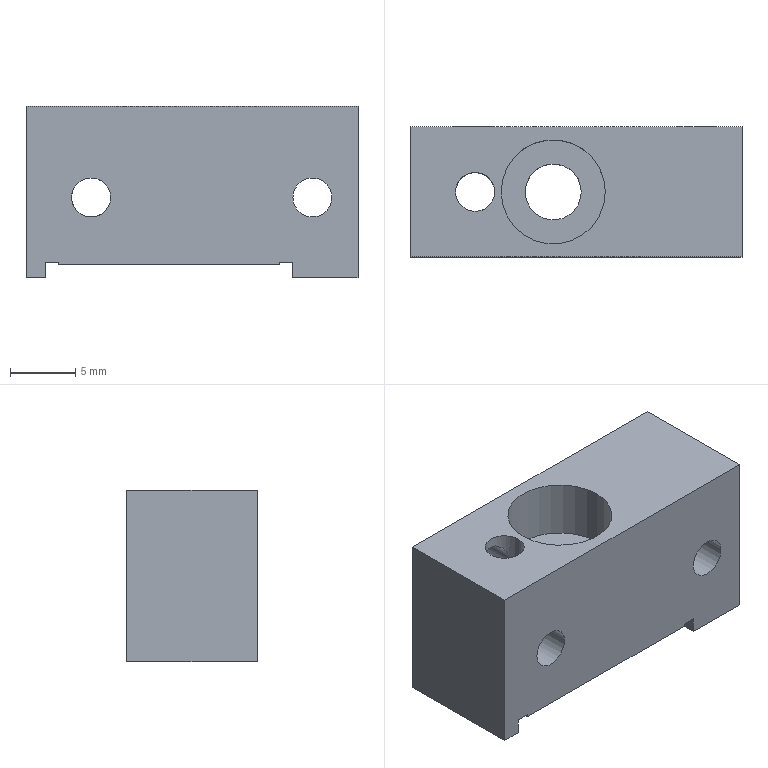Part | NX | 1 solid | 33 faces | box 25.5 x 10 x 13.2 mm | volume 2606 mm3 | cylinder 16 | plane 15 | cone 2 | commonest cylinder face diameters 3 x10 2.5 x2 4.3 x2 8 x2
STEP:
#1=CARTESIAN_POINT('',(9.5,5.,-6.6));
#2=VERTEX_POINT('',#1);
#3=CARTESIAN_POINT('',(9.5,-5.,-6.6));
#4=VERTEX_POINT('',#3);
#5=CARTESIAN_POINT('',(9.5,0.,-6.6));
#6=DIRECTION('',(0.,-1.,0.));
#7=VECTOR('',#6,1000.);
#8=LINE('',#5,#7);
#9=EDGE_CURVE('',#2,#4,#8,.T.);
#10=ORIENTED_EDGE('',*,*,#9,.F.);
#11=CARTESIAN_POINT('',(14.5,5.,-6.6));
#12=VERTEX_POINT('',#11);
#13=CARTESIAN_POINT('',(0.,5.,-6.6));
#14=DIRECTION('',(-1.,0.,0.));
#15=VECTOR('',#14,1000.);
#16=LINE('',#13,#15);
#17=EDGE_CURVE('',#12,#2,#16,.T.);
#18=ORIENTED_EDGE('',*,*,#17,.F.);
#19=CARTESIAN_POINT('',(14.5,-5.,-6.6));
#20=VERTEX_POINT('',#19);
#21=CARTESIAN_POINT('',(14.5,0.,-6.6));
#22=DIRECTION('',(0.,1.,0.));
#23=VECTOR('',#22,1000.);
#24=LINE('',#21,#23);
#25=EDGE_CURVE('',#20,#12,#24,.T.);
#26=ORIENTED_EDGE('',*,*,#25,.F.);
#27=CARTESIAN_POINT('',(0.,-5.,-6.6));
#28=DIRECTION('',(1.,0.,0.));
#29=VECTOR('',#28,1000.);
#30=LINE('',#27,#29);
#31=EDGE_CURVE('',#4,#20,#30,.T.);
#32=ORIENTED_EDGE('',*,*,#31,.F.);
#33=EDGE_LOOP('',(#10,#18,#26,#32));
#34=FACE_BOUND('',#33,.T.);
#35=CARTESIAN_POINT('',(0.,0.,-6.6));
#36=DIRECTION('',(0.,0.,1.));
#37=DIRECTION('',(1.,0.,0.));
#38=AXIS2_PLACEMENT_3D('',#35,#36,#37);
#39=PLANE('',#38);
#40=ADVANCED_FACE('',(#34),#39,.F.);
#41=CARTESIAN_POINT('',(9.5,5.,-5.4));
#42=VERTEX_POINT('',#41);
#43=CARTESIAN_POINT('',(9.5,5.,0.));
#44=DIRECTION('',(0.,0.,1.));
#45=VECTOR('',#44,1000.);
#46=LINE('',#43,#45);
#47=EDGE_CURVE('',#2,#42,#46,.T.);
#48=ORIENTED_EDGE('',*,*,#47,.F.);
#49=ORIENTED_EDGE('',*,*,#9,.T.);
#50=CARTESIAN_POINT('',(9.5,-5.,-5.4));
#51=VERTEX_POINT('',#50);
#52=CARTESIAN_POINT('',(9.5,-5.,0.));
#53=DIRECTION('',(0.,0.,-1.));
#54=VECTOR('',#53,1000.);
#55=LINE('',#52,#54);
#56=EDGE_CURVE('',#51,#4,#55,.T.);
#57=ORIENTED_EDGE('',*,*,#56,.F.);
#58=CARTESIAN_POINT('',(9.5,5.,-5.4));
#59=DIRECTION('',(0.,-1.,0.));
#60=VECTOR('',#59,1000.);
#61=LINE('',#58,#60);
#62=EDGE_CURVE('',#42,#51,#61,.T.);
#63=ORIENTED_EDGE('',*,*,#62,.F.);
#64=EDGE_LOOP('',(#48,#49,#57,#63));
#65=FACE_BOUND('',#64,.T.);
#66=CARTESIAN_POINT('',(9.5,-5.,-6.6));
#67=DIRECTION('',(1.,0.,0.));
#68=DIRECTION('',(0.,1.,0.));
#69=AXIS2_PLACEMENT_3D('',#66,#67,#68);
#70=PLANE('',#69);
#71=ADVANCED_FACE('',(#65),#70,.F.);
#72=CARTESIAN_POINT('',(-11.,-5.,6.6));
#73=VERTEX_POINT('',#72);
#74=CARTESIAN_POINT('',(-11.,5.,6.6));
#75=VERTEX_POINT('',#74);
#76=CARTESIAN_POINT('',(-11.,0.,6.6));
#77=DIRECTION('',(0.,1.,0.));
#78=VECTOR('',#77,1000.);
#79=LINE('',#76,#78);
#80=EDGE_CURVE('',#73,#75,#79,.T.);
#81=ORIENTED_EDGE('',*,*,#80,.F.);
#82=CARTESIAN_POINT('',(14.5,-5.,6.6));
#83=VERTEX_POINT('',#82);
#84=CARTESIAN_POINT('',(0.,-5.,6.6));
#85=DIRECTION('',(-1.,0.,0.));
#86=VECTOR('',#85,1000.);
#87=LINE('',#84,#86);
#88=EDGE_CURVE('',#83,#73,#87,.T.);
#89=ORIENTED_EDGE('',*,*,#88,.F.);
#90=CARTESIAN_POINT('',(14.5,5.,6.6));
#91=VERTEX_POINT('',#90);
#92=CARTESIAN_POINT('',(14.5,0.,6.6));
#93=DIRECTION('',(0.,-1.,0.));
#94=VECTOR('',#93,1000.);
#95=LINE('',#92,#94);
#96=EDGE_CURVE('',#91,#83,#95,.T.);
#97=ORIENTED_EDGE('',*,*,#96,.F.);
#98=CARTESIAN_POINT('',(0.,5.,6.6));
#99=DIRECTION('',(-1.,0.,0.));
#100=VECTOR('',#99,1000.);
#101=LINE('',#98,#100);
#102=EDGE_CURVE('',#91,#75,#101,.T.);
#103=ORIENTED_EDGE('',*,*,#102,.T.);
#104=EDGE_LOOP('',(#81,#89,#97,#103));
#105=FACE_BOUND('',#104,.T.);
#106=CARTESIAN_POINT('',(4.,0.,6.6));
#107=VERTEX_POINT('',#106);
#108=CARTESIAN_POINT('',(-4.,0.,6.6));
#109=VERTEX_POINT('',#108);
#110=CARTESIAN_POINT('',(0.,0.,6.6));
#111=DIRECTION('',(0.,0.,1.));
#112=DIRECTION('',(-1.,0.,0.));
#113=AXIS2_PLACEMENT_3D('',#110,#111,#112);
#114=CIRCLE('',#113,4.);
#115=EDGE_CURVE('',#107,#109,#114,.T.);
#116=ORIENTED_EDGE('',*,*,#115,.F.);
#117=CARTESIAN_POINT('',(0.,0.,6.6));
#118=DIRECTION('',(0.,0.,1.));
#119=DIRECTION('',(-1.,0.,0.));
#120=AXIS2_PLACEMENT_3D('',#117,#118,#119);
#121=CIRCLE('',#120,4.);
#122=EDGE_CURVE('',#109,#107,#121,.T.);
#123=ORIENTED_EDGE('',*,*,#122,.F.);
#124=EDGE_LOOP('',(#116,#123));
#125=FACE_BOUND('',#124,.T.);
#126=CARTESIAN_POINT('',(-4.5,0.,6.6));
#127=VERTEX_POINT('',#126);
#128=CARTESIAN_POINT('',(-7.5,0.,6.6));
#129=VERTEX_POINT('',#128);
#130=CARTESIAN_POINT('',(-6.,0.,6.6));
#131=DIRECTION('',(0.,0.,-1.));
#132=DIRECTION('',(-1.,0.,0.));
#133=AXIS2_PLACEMENT_3D('',#130,#131,#132);
#134=CIRCLE('',#133,1.5);
#135=EDGE_CURVE('',#127,#129,#134,.T.);
#136=ORIENTED_EDGE('',*,*,#135,.T.);
#137=CARTESIAN_POINT('',(-6.,0.,6.6));
#138=DIRECTION('',(0.,0.,-1.));
#139=DIRECTION('',(-1.,0.,0.));
#140=AXIS2_PLACEMENT_3D('',#137,#138,#139);
#141=CIRCLE('',#140,1.5);
#142=EDGE_CURVE('',#129,#127,#141,.T.);
#143=ORIENTED_EDGE('',*,*,#142,.T.);
#144=EDGE_LOOP('',(#136,#143));
#145=FACE_BOUND('',#144,.T.);
#146=CARTESIAN_POINT('',(0.,0.,6.6));
#147=DIRECTION('',(0.,0.,1.));
#148=DIRECTION('',(1.,0.,0.));
#149=AXIS2_PLACEMENT_3D('',#146,#147,#148);
#150=PLANE('',#149);
#151=ADVANCED_FACE('',(#105,#125,#145),#150,.T.);
#152=CARTESIAN_POINT('',(8.5,-5.,-5.4));
#153=VERTEX_POINT('',#152);
#154=CARTESIAN_POINT('',(0.,-5.,-5.4));
#155=DIRECTION('',(1.,0.,0.));
#156=VECTOR('',#155,1000.);
#157=LINE('',#154,#156);
#158=EDGE_CURVE('',#153,#51,#157,.T.);
#159=ORIENTED_EDGE('',*,*,#158,.F.);
#160=CARTESIAN_POINT('',(8.5,5.,-5.4));
#161=VERTEX_POINT('',#160);
#162=CARTESIAN_POINT('',(8.5,5.,-5.4));
#163=DIRECTION('',(0.,-1.,0.));
#164=VECTOR('',#163,1000.);
#165=LINE('',#162,#164);
#166=EDGE_CURVE('',#161,#153,#165,.T.);
#167=ORIENTED_EDGE('',*,*,#166,.F.);
#168=CARTESIAN_POINT('',(0.,5.,-5.4));
#169=DIRECTION('',(-1.,0.,0.));
#170=VECTOR('',#169,1000.);
#171=LINE('',#168,#170);
#172=EDGE_CURVE('',#42,#161,#171,.T.);
#173=ORIENTED_EDGE('',*,*,#172,.F.);
#174=ORIENTED_EDGE('',*,*,#62,.T.);
#175=EDGE_LOOP('',(#159,#167,#173,#174));
#176=FACE_BOUND('',#175,.T.);
#177=CARTESIAN_POINT('',(9.5,-5.,-5.4));
#178=DIRECTION('',(0.,0.,1.));
#179=DIRECTION('',(1.,0.,0.));
#180=AXIS2_PLACEMENT_3D('',#177,#178,#179);
#181=PLANE('',#180);
#182=ADVANCED_FACE('',(#176),#181,.F.);
#183=CARTESIAN_POINT('',(-7.5,0.,-0.42));
#184=VERTEX_POINT('',#183);
#185=CARTESIAN_POINT('',(-4.5,0.,-0.42));
#186=VERTEX_POINT('',#185);
#187=CARTESIAN_POINT('',(-7.5,0.,-0.42));
#188=CARTESIAN_POINT('',(-7.5,3.,-3.42));
#189=CARTESIAN_POINT('',(-4.5,3.,-3.42));
#190=CARTESIAN_POINT('',(-4.5,0.,-0.42));
#191=(BOUNDED_CURVE()B_SPLINE_CURVE(3,(#187,#188,#189,#190),.UNSPECIFIED.,.F.,.F.)B_SPLINE_CURVE_WITH_KNOTS((4,4),(4.712,7.854),.UNSPECIFIED.)CURVE()GEOMETRIC_REPRESENTATION_ITEM()RATIONAL_B_SPLINE_CURVE((1.,0.3333,0.3333,1.))REPRESENTATION_ITEM(''));
#192=EDGE_CURVE('',#184,#186,#191,.T.);
#193=ORIENTED_EDGE('',*,*,#192,.F.);
#194=CARTESIAN_POINT('',(-7.5,0.,-5.6));
#195=VERTEX_POINT('',#194);
#196=CARTESIAN_POINT('',(-7.5,0.,6.6));
#197=DIRECTION('',(0.,0.,-1.));
#198=VECTOR('',#197,1000.);
#199=LINE('',#196,#198);
#200=EDGE_CURVE('',#195,#184,#199,.F.);
#201=ORIENTED_EDGE('',*,*,#200,.F.);
#202=CARTESIAN_POINT('',(-4.5,0.,-5.6));
#203=VERTEX_POINT('',#202);
#204=CARTESIAN_POINT('',(-6.,0.,-5.6));
#205=DIRECTION('',(0.,0.,-1.));
#206=DIRECTION('',(-1.,0.,0.));
#207=AXIS2_PLACEMENT_3D('',#204,#205,#206);
#208=CIRCLE('',#207,1.5);
#209=EDGE_CURVE('',#195,#203,#208,.T.);
#210=ORIENTED_EDGE('',*,*,#209,.T.);
#211=CARTESIAN_POINT('',(-4.5,0.,6.6));
#212=DIRECTION('',(0.,0.,-1.));
#213=VECTOR('',#212,1000.);
#214=LINE('',#211,#213);
#215=EDGE_CURVE('',#203,#186,#214,.F.);
#216=ORIENTED_EDGE('',*,*,#215,.T.);
#217=EDGE_LOOP('',(#193,#201,#210,#216));
#218=FACE_BOUND('',#217,.T.);
#219=CARTESIAN_POINT('',(-6.,0.,6.6));
#220=DIRECTION('',(0.,0.,-1.));
#221=DIRECTION('',(-1.,0.,0.));
#222=AXIS2_PLACEMENT_3D('',#219,#220,#221);
#223=CYLINDRICAL_SURFACE('',#222,1.5);
#224=ADVANCED_FACE('',(#218),#223,.F.);
#225=CARTESIAN_POINT('',(-4.5,5.,-0.42));
#226=VERTEX_POINT('',#225);
#227=CARTESIAN_POINT('',(-7.5,5.,-0.42));
#228=VERTEX_POINT('',#227);
#229=CARTESIAN_POINT('',(-6.,5.,-0.42));
#230=DIRECTION('',(0.,1.,0.));
#231=DIRECTION('',(-1.,0.,0.));
#232=AXIS2_PLACEMENT_3D('',#229,#230,#231);
#233=CIRCLE('',#232,1.5);
#234=EDGE_CURVE('',#226,#228,#233,.T.);
#235=ORIENTED_EDGE('',*,*,#234,.T.);
#236=CARTESIAN_POINT('',(-7.5,-5.,-0.42));
#237=DIRECTION('',(0.,1.,0.));
#238=VECTOR('',#237,1000.);
#239=LINE('',#236,#238);
#240=EDGE_CURVE('',#228,#184,#239,.F.);
#241=ORIENTED_EDGE('',*,*,#240,.T.);
#242=ORIENTED_EDGE('',*,*,#192,.T.);
#243=CARTESIAN_POINT('',(-4.5,-5.,-0.42));
#244=DIRECTION('',(0.,1.,0.));
#245=VECTOR('',#244,1000.);
#246=LINE('',#243,#245);
#247=EDGE_CURVE('',#226,#186,#246,.F.);
#248=ORIENTED_EDGE('',*,*,#247,.F.);
#249=EDGE_LOOP('',(#235,#241,#242,#248));
#250=FACE_BOUND('',#249,.T.);
#251=CARTESIAN_POINT('',(-6.,-5.,-0.42));
#252=DIRECTION('',(0.,1.,0.));
#253=DIRECTION('',(-1.,0.,0.));
#254=AXIS2_PLACEMENT_3D('',#251,#252,#253);
#255=CYLINDRICAL_SURFACE('',#254,1.5);
#256=ADVANCED_FACE('',(#250),#255,.F.);
#257=CARTESIAN_POINT('',(9.5,-5.,-0.42));
#258=VERTEX_POINT('',#257);
#259=CARTESIAN_POINT('',(12.5,-5.,-0.42));
#260=VERTEX_POINT('',#259);
#261=CARTESIAN_POINT('',(11.,-5.,-0.42));
#262=DIRECTION('',(0.,1.,0.));
#263=DIRECTION('',(-1.,0.,0.));
#264=AXIS2_PLACEMENT_3D('',#261,#262,#263);
#265=CIRCLE('',#264,1.5);
#266=EDGE_CURVE('',#258,#260,#265,.T.);
#267=ORIENTED_EDGE('',*,*,#266,.F.);
#268=CARTESIAN_POINT('',(9.5,5.,-0.42));
#269=VERTEX_POINT('',#268);
#270=CARTESIAN_POINT('',(9.5,-5.,-0.42));
#271=DIRECTION('',(0.,1.,0.));
#272=VECTOR('',#271,1000.);
#273=LINE('',#270,#272);
#274=EDGE_CURVE('',#269,#258,#273,.F.);
#275=ORIENTED_EDGE('',*,*,#274,.F.);
#276=CARTESIAN_POINT('',(12.5,5.,-0.42));
#277=VERTEX_POINT('',#276);
#278=CARTESIAN_POINT('',(11.,5.,-0.42));
#279=DIRECTION('',(0.,1.,0.));
#280=DIRECTION('',(-1.,0.,0.));
#281=AXIS2_PLACEMENT_3D('',#278,#279,#280);
#282=CIRCLE('',#281,1.5);
#283=EDGE_CURVE('',#269,#277,#282,.T.);
#284=ORIENTED_EDGE('',*,*,#283,.T.);
#285=CARTESIAN_POINT('',(12.5,-5.,-0.42));
#286=DIRECTION('',(0.,1.,0.));
#287=VECTOR('',#286,1000.);
#288=LINE('',#285,#287);
#289=EDGE_CURVE('',#277,#260,#288,.F.);
#290=ORIENTED_EDGE('',*,*,#289,.T.);
#291=EDGE_LOOP('',(#267,#275,#284,#290));
#292=FACE_BOUND('',#291,.T.);
#293=CARTESIAN_POINT('',(11.,-5.,-0.42));
#294=DIRECTION('',(0.,1.,0.));
#295=DIRECTION('',(-1.,0.,0.));
#296=AXIS2_PLACEMENT_3D('',#293,#294,#295);
#297=CYLINDRICAL_SURFACE('',#296,1.5);
#298=ADVANCED_FACE('',(#292),#297,.F.);
#299=ORIENTED_EDGE('',*,*,#135,.F.);
#300=CARTESIAN_POINT('',(-4.5,0.,6.6));
#301=DIRECTION('',(0.,0.,-1.));
#302=VECTOR('',#301,1000.);
#303=LINE('',#300,#302);
#304=EDGE_CURVE('',#186,#127,#303,.F.);
#305=ORIENTED_EDGE('',*,*,#304,.F.);
#306=CARTESIAN_POINT('',(-7.5,0.,-0.42));
#307=CARTESIAN_POINT('',(-7.5,-3.,2.58));
#308=CARTESIAN_POINT('',(-4.5,-3.,2.58));
#309=CARTESIAN_POINT('',(-4.5,0.,-0.42));
#310=(BOUNDED_CURVE()B_SPLINE_CURVE(3,(#306,#307,#308,#309),.UNSPECIFIED.,.F.,.F.)B_SPLINE_CURVE_WITH_KNOTS((4,4),(1.571,4.712),.UNSPECIFIED.)CURVE()GEOMETRIC_REPRESENTATION_ITEM()RATIONAL_B_SPLINE_CURVE((1.,0.3333,0.3333,1.))REPRESENTATION_ITEM(''));
#311=EDGE_CURVE('',#184,#186,#310,.T.);
#312=ORIENTED_EDGE('',*,*,#311,.F.);
#313=CARTESIAN_POINT('',(-7.5,0.,6.6));
#314=DIRECTION('',(0.,0.,-1.));
#315=VECTOR('',#314,1000.);
#316=LINE('',#313,#315);
#317=EDGE_CURVE('',#184,#129,#316,.F.);
#318=ORIENTED_EDGE('',*,*,#317,.T.);
#319=EDGE_LOOP('',(#299,#305,#312,#318));
#320=FACE_BOUND('',#319,.T.);
#321=CARTESIAN_POINT('',(-6.,0.,6.6));
#322=DIRECTION('',(0.,0.,-1.));
#323=DIRECTION('',(-1.,0.,0.));
#324=AXIS2_PLACEMENT_3D('',#321,#322,#323);
#325=CYLINDRICAL_SURFACE('',#324,1.5);
#326=ADVANCED_FACE('',(#320),#325,.F.);
#327=CARTESIAN_POINT('',(-8.5,-5.,-5.6));
#328=VERTEX_POINT('',#327);
#329=CARTESIAN_POINT('',(8.5,-5.,-5.6));
#330=VERTEX_POINT('',#329);
#331=CARTESIAN_POINT('',(0.,-5.,-5.6));
#332=DIRECTION('',(1.,0.,0.));
#333=VECTOR('',#332,1000.);
#334=LINE('',#331,#333);
#335=EDGE_CURVE('',#328,#330,#334,.T.);
#336=ORIENTED_EDGE('',*,*,#335,.T.);
#337=CARTESIAN_POINT('',(8.5,-5.,0.));
#338=DIRECTION('',(0.,0.,1.));
#339=VECTOR('',#338,1000.);
#340=LINE('',#337,#339);
#341=EDGE_CURVE('',#330,#153,#340,.T.);
#342=ORIENTED_EDGE('',*,*,#341,.T.);
#343=ORIENTED_EDGE('',*,*,#158,.T.);
#344=ORIENTED_EDGE('',*,*,#56,.T.);
#345=ORIENTED_EDGE('',*,*,#31,.T.);
#346=CARTESIAN_POINT('',(14.5,-5.,0.));
#347=DIRECTION('',(0.,0.,-1.));
#348=VECTOR('',#347,1000.);
#349=LINE('',#346,#348);
#350=EDGE_CURVE('',#83,#20,#349,.T.);
#351=ORIENTED_EDGE('',*,*,#350,.F.);
#352=ORIENTED_EDGE('',*,*,#88,.T.);
#353=CARTESIAN_POINT('',(-11.,-5.,-6.6));
#354=VERTEX_POINT('',#353);
#355=CARTESIAN_POINT('',(-11.,-5.,0.));
#356=DIRECTION('',(0.,0.,1.));
#357=VECTOR('',#356,1000.);
#358=LINE('',#355,#357);
#359=EDGE_CURVE('',#354,#73,#358,.T.);
#360=ORIENTED_EDGE('',*,*,#359,.F.);
#361=CARTESIAN_POINT('',(-9.5,-5.,-6.6));
#362=VERTEX_POINT('',#361);
#363=CARTESIAN_POINT('',(0.,-5.,-6.6));
#364=DIRECTION('',(1.,0.,0.));
#365=VECTOR('',#364,1000.);
#366=LINE('',#363,#365);
#367=EDGE_CURVE('',#354,#362,#366,.T.);
#368=ORIENTED_EDGE('',*,*,#367,.T.);
#369=CARTESIAN_POINT('',(-9.5,-5.,-5.4));
#370=VERTEX_POINT('',#369);
#371=CARTESIAN_POINT('',(-9.5,-5.,0.));
#372=DIRECTION('',(0.,0.,1.));
#373=VECTOR('',#372,1000.);
#374=LINE('',#371,#373);
#375=EDGE_CURVE('',#362,#370,#374,.T.);
#376=ORIENTED_EDGE('',*,*,#375,.T.);
#377=CARTESIAN_POINT('',(-8.5,-5.,-5.4));
#378=VERTEX_POINT('',#377);
#379=CARTESIAN_POINT('',(0.,-5.,-5.4));
#380=DIRECTION('',(1.,0.,0.));
#381=VECTOR('',#380,1000.);
#382=LINE('',#379,#381);
#383=EDGE_CURVE('',#370,#378,#382,.T.);
#384=ORIENTED_EDGE('',*,*,#383,.T.);
#385=CARTESIAN_POINT('',(-8.5,-5.,0.));
#386=DIRECTION('',(0.,0.,-1.));
#387=VECTOR('',#386,1000.);
#388=LINE('',#385,#387);
#389=EDGE_CURVE('',#378,#328,#388,.T.);
#390=ORIENTED_EDGE('',*,*,#389,.T.);
#391=EDGE_LOOP('',(#336,#342,#343,#344,#345,#351,#352,#360,#368,#376,#384,#390));
#392=FACE_BOUND('',#391,.T.);
#393=CARTESIAN_POINT('',(-4.5,-5.,-0.42));
#394=VERTEX_POINT('',#393);
#395=CARTESIAN_POINT('',(-7.5,-5.,-0.42));
#396=VERTEX_POINT('',#395);
#397=CARTESIAN_POINT('',(-6.,-5.,-0.42));
#398=DIRECTION('',(0.,1.,0.));
#399=DIRECTION('',(-1.,0.,0.));
#400=AXIS2_PLACEMENT_3D('',#397,#398,#399);
#401=CIRCLE('',#400,1.5);
#402=EDGE_CURVE('',#394,#396,#401,.T.);
#403=ORIENTED_EDGE('',*,*,#402,.T.);
#404=CARTESIAN_POINT('',(-6.,-5.,-0.42));
#405=DIRECTION('',(0.,1.,0.));
#406=DIRECTION('',(-1.,0.,0.));
#407=AXIS2_PLACEMENT_3D('',#404,#405,#406);
#408=CIRCLE('',#407,1.5);
#409=EDGE_CURVE('',#396,#394,#408,.T.);
#410=ORIENTED_EDGE('',*,*,#409,.T.);
#411=EDGE_LOOP('',(#403,#410));
#412=FACE_BOUND('',#411,.T.);
#413=ORIENTED_EDGE('',*,*,#266,.T.);
#414=CARTESIAN_POINT('',(11.,-5.,-0.42));
#415=DIRECTION('',(0.,1.,0.));
#416=DIRECTION('',(-1.,0.,0.));
#417=AXIS2_PLACEMENT_3D('',#414,#415,#416);
#418=CIRCLE('',#417,1.5);
#419=EDGE_CURVE('',#260,#258,#418,.T.);
#420=ORIENTED_EDGE('',*,*,#419,.T.);
#421=EDGE_LOOP('',(#413,#420));
#422=FACE_BOUND('',#421,.T.);
#423=CARTESIAN_POINT('',(-11.,-5.,-6.6));
#424=DIRECTION('',(0.,-1.,0.));
#425=DIRECTION('',(0.,0.,-1.));
#426=AXIS2_PLACEMENT_3D('',#423,#424,#425);
#427=PLANE('',#426);
#428=ADVANCED_FACE('',(#392,#412,#422),#427,.T.);
#429=CARTESIAN_POINT('',(-11.,5.,-6.6));
#430=VERTEX_POINT('',#429);
#431=CARTESIAN_POINT('',(-11.,-5.,-6.6));
#432=DIRECTION('',(0.,1.,0.));
#433=VECTOR('',#432,1000.);
#434=LINE('',#431,#433);
#435=EDGE_CURVE('',#354,#430,#434,.T.);
#436=ORIENTED_EDGE('',*,*,#435,.F.);
#437=ORIENTED_EDGE('',*,*,#359,.T.);
#438=ORIENTED_EDGE('',*,*,#80,.T.);
#439=CARTESIAN_POINT('',(-11.,5.,0.));
#440=DIRECTION('',(0.,0.,-1.));
#441=VECTOR('',#440,1000.);
#442=LINE('',#439,#441);
#443=EDGE_CURVE('',#75,#430,#442,.T.);
#444=ORIENTED_EDGE('',*,*,#443,.T.);
#445=EDGE_LOOP('',(#436,#437,#438,#444));
#446=FACE_BOUND('',#445,.T.);
#447=CARTESIAN_POINT('',(-11.,5.,-6.6));
#448=DIRECTION('',(-1.,0.,0.));
#449=DIRECTION('',(0.,0.,1.));
#450=AXIS2_PLACEMENT_3D('',#447,#448,#449);
#451=PLANE('',#450);
#452=ADVANCED_FACE('',(#446),#451,.T.);
#453=CARTESIAN_POINT('',(-9.5,5.,-6.6));
#454=VERTEX_POINT('',#453);
#455=CARTESIAN_POINT('',(-9.5,0.,-6.6));
#456=DIRECTION('',(0.,-1.,0.));
#457=VECTOR('',#456,1000.);
#458=LINE('',#455,#457);
#459=EDGE_CURVE('',#454,#362,#458,.T.);
#460=ORIENTED_EDGE('',*,*,#459,.T.);
#461=ORIENTED_EDGE('',*,*,#367,.F.);
#462=ORIENTED_EDGE('',*,*,#435,.T.);
#463=CARTESIAN_POINT('',(0.,5.,-6.6));
#464=DIRECTION('',(-1.,0.,0.));
#465=VECTOR('',#464,1000.);
#466=LINE('',#463,#465);
#467=EDGE_CURVE('',#454,#430,#466,.T.);
#468=ORIENTED_EDGE('',*,*,#467,.F.);
#469=EDGE_LOOP('',(#460,#461,#462,#468));
#470=FACE_BOUND('',#469,.T.);
#471=CARTESIAN_POINT('',(0.,0.,-6.6));
#472=DIRECTION('',(0.,0.,1.));
#473=DIRECTION('',(1.,0.,0.));
#474=AXIS2_PLACEMENT_3D('',#471,#472,#473);
#475=PLANE('',#474);
#476=ADVANCED_FACE('',(#470),#475,.F.);
#477=ORIENTED_EDGE('',*,*,#375,.F.);
#478=ORIENTED_EDGE('',*,*,#459,.F.);
#479=CARTESIAN_POINT('',(-9.5,5.,-5.4));
#480=VERTEX_POINT('',#479);
#481=CARTESIAN_POINT('',(-9.5,5.,0.));
#482=DIRECTION('',(0.,0.,-1.));
#483=VECTOR('',#482,1000.);
#484=LINE('',#481,#483);
#485=EDGE_CURVE('',#480,#454,#484,.T.);
#486=ORIENTED_EDGE('',*,*,#485,.F.);
#487=CARTESIAN_POINT('',(-9.5,6.,-5.4));
#488=DIRECTION('',(0.,-1.,0.));
#489=VECTOR('',#488,1000.);
#490=LINE('',#487,#489);
#491=EDGE_CURVE('',#480,#370,#490,.T.);
#492=ORIENTED_EDGE('',*,*,#491,.T.);
#493=EDGE_LOOP('',(#477,#478,#486,#492));
#494=FACE_BOUND('',#493,.T.);
#495=CARTESIAN_POINT('',(-9.5,-5.,-5.6));
#496=DIRECTION('',(-1.,0.,0.));
#497=DIRECTION('',(0.,0.,1.));
#498=AXIS2_PLACEMENT_3D('',#495,#496,#497);
#499=PLANE('',#498);
#500=ADVANCED_FACE('',(#494),#499,.F.);
#501=CARTESIAN_POINT('',(-8.5,5.,-5.6));
#502=VERTEX_POINT('',#501);
#503=CARTESIAN_POINT('',(-8.5,0.,-5.6));
#504=DIRECTION('',(0.,-1.,0.));
#505=VECTOR('',#504,1000.);
#506=LINE('',#503,#505);
#507=EDGE_CURVE('',#502,#328,#506,.T.);
#508=ORIENTED_EDGE('',*,*,#507,.F.);
#509=CARTESIAN_POINT('',(8.5,5.,-5.6));
#510=VERTEX_POINT('',#509);
#511=CARTESIAN_POINT('',(0.,5.,-5.6));
#512=DIRECTION('',(-1.,0.,0.));
#513=VECTOR('',#512,1000.);
#514=LINE('',#511,#513);
#515=EDGE_CURVE('',#510,#502,#514,.T.);
#516=ORIENTED_EDGE('',*,*,#515,.F.);
#517=CARTESIAN_POINT('',(8.5,0.,-5.6));
#518=DIRECTION('',(0.,1.,0.));
#519=VECTOR('',#518,1000.);
#520=LINE('',#517,#519);
#521=EDGE_CURVE('',#330,#510,#520,.T.);
#522=ORIENTED_EDGE('',*,*,#521,.F.);
#523=ORIENTED_EDGE('',*,*,#335,.F.);
#524=EDGE_LOOP('',(#508,#516,#522,#523));
#525=FACE_BOUND('',#524,.T.);
#526=CARTESIAN_POINT('',(2.15,0.,-5.6));
#527=VERTEX_POINT('',#526);
#528=CARTESIAN_POINT('',(-2.15,0.,-5.6));
#529=VERTEX_POINT('',#528);
#530=CARTESIAN_POINT('',(0.,0.,-5.6));
#531=DIRECTION('',(0.,0.,1.));
#532=DIRECTION('',(-1.,0.,0.));
#533=AXIS2_PLACEMENT_3D('',#530,#531,#532);
#534=CIRCLE('',#533,2.15);
#535=EDGE_CURVE('',#527,#529,#534,.T.);
#536=ORIENTED_EDGE('',*,*,#535,.T.);
#537=CARTESIAN_POINT('',(0.,0.,-5.6));
#538=DIRECTION('',(0.,0.,1.));
#539=DIRECTION('',(-1.,0.,0.));
#540=AXIS2_PLACEMENT_3D('',#537,#538,#539);
#541=CIRCLE('',#540,2.15);
#542=EDGE_CURVE('',#529,#527,#541,.T.);
#543=ORIENTED_EDGE('',*,*,#542,.T.);
#544=EDGE_LOOP('',(#536,#543));
#545=FACE_BOUND('',#544,.T.);
#546=CARTESIAN_POINT('',(-6.,0.,-5.6));
#547=DIRECTION('',(0.,0.,-1.));
#548=DIRECTION('',(-1.,0.,0.));
#549=AXIS2_PLACEMENT_3D('',#546,#547,#548);
#550=CIRCLE('',#549,1.5);
#551=EDGE_CURVE('',#203,#195,#550,.T.);
#552=ORIENTED_EDGE('',*,*,#551,.F.);
#553=ORIENTED_EDGE('',*,*,#209,.F.);
#554=EDGE_LOOP('',(#552,#553));
#555=FACE_BOUND('',#554,.T.);
#556=CARTESIAN_POINT('',(9.5,-5.,-5.6));
#557=DIRECTION('',(0.,0.,1.));
#558=DIRECTION('',(1.,0.,0.));
#559=AXIS2_PLACEMENT_3D('',#556,#557,#558);
#560=PLANE('',#559);
#561=ADVANCED_FACE('',(#525,#545,#555),#560,.F.);
#562=CARTESIAN_POINT('',(-4.75,0.8292,4.6));
#563=VERTEX_POINT('',#562);
#564=CARTESIAN_POINT('',(-7.25,0.8292,4.6));
#565=VERTEX_POINT('',#564);
#566=CARTESIAN_POINT('',(-4.75,0.8292,4.6));
#567=CARTESIAN_POINT('',(-4.75,0.8292,4.766));
#568=CARTESIAN_POINT('',(-4.828,0.9361,5.054));
#569=CARTESIAN_POINT('',(-4.907,1.037,5.23));
#570=CARTESIAN_POINT('',(-5.078,1.185,5.448));
#571=CARTESIAN_POINT('',(-5.098,1.2,5.467));
#572=CARTESIAN_POINT('',(-5.321,1.346,5.664));
#573=CARTESIAN_POINT('',(-5.543,1.438,5.773));
#574=CARTESIAN_POINT('',(-6.,1.542,5.901));
#575=CARTESIAN_POINT('',(-6.457,1.438,5.774));
#576=CARTESIAN_POINT('',(-6.68,1.345,5.663));
#577=CARTESIAN_POINT('',(-6.9,1.202,5.47));
#578=CARTESIAN_POINT('',(-6.925,1.182,5.444));
#579=CARTESIAN_POINT('',(-7.09,1.039,5.233));
#580=CARTESIAN_POINT('',(-7.174,0.9344,5.052));
#581=CARTESIAN_POINT('',(-7.25,0.8292,4.766));
#582=CARTESIAN_POINT('',(-7.25,0.8292,4.6));
#583=B_SPLINE_CURVE_WITH_KNOTS('',3,(#566,#567,#568,#569,#570,#571,#572,#573,#574,#575,#576,#577,#578,#579,#580,#581,#582),.UNSPECIFIED.,.F.,.F.,(4,1,1,1,1,1,1,1,1,1,1,1,1,1,4),(0.,0.125,0.1875,0.2188,0.25,0.3125,0.375,0.5,0.625,0.6875,0.75,0.7812,0.8125,0.875,1.),.UNSPECIFIED.);
#584=EDGE_CURVE('',#563,#565,#583,.T.);
#585=ORIENTED_EDGE('',*,*,#584,.T.);
#586=CARTESIAN_POINT('',(-7.25,4.74,4.6));
#587=VERTEX_POINT('',#586);
#588=CARTESIAN_POINT('',(-7.25,2.915,4.6));
#589=DIRECTION('',(0.,1.,0.));
#590=VECTOR('',#589,1000.);
#591=LINE('',#588,#590);
#592=EDGE_CURVE('',#587,#565,#591,.F.);
#593=ORIENTED_EDGE('',*,*,#592,.F.);
#594=CARTESIAN_POINT('',(-4.75,4.74,4.6));
#595=VERTEX_POINT('',#594);
#596=CARTESIAN_POINT('',(-6.,4.74,4.6));
#597=DIRECTION('',(0.,1.,0.));
#598=DIRECTION('',(1.,0.,0.));
#599=AXIS2_PLACEMENT_3D('',#596,#597,#598);
#600=CIRCLE('',#599,1.25);
#601=EDGE_CURVE('',#587,#595,#600,.T.);
#602=ORIENTED_EDGE('',*,*,#601,.T.);
#603=CARTESIAN_POINT('',(-4.75,2.915,4.6));
#604=DIRECTION('',(0.,1.,0.));
#605=VECTOR('',#604,1000.);
#606=LINE('',#603,#605);
#607=EDGE_CURVE('',#595,#563,#606,.F.);
#608=ORIENTED_EDGE('',*,*,#607,.T.);
#609=EDGE_LOOP('',(#585,#593,#602,#608));
#610=FACE_BOUND('',#609,.T.);
#611=CARTESIAN_POINT('',(-6.,2.915,4.6));
#612=DIRECTION('',(0.,1.,0.));
#613=DIRECTION('',(-1.,0.,0.));
#614=AXIS2_PLACEMENT_3D('',#611,#612,#613);
#615=CYLINDRICAL_SURFACE('',#614,1.25);
#616=ADVANCED_FACE('',(#610),#615,.F.);
#617=ORIENTED_EDGE('',*,*,#115,.T.);
#618=CARTESIAN_POINT('',(-4.,0.,2.1));
#619=VERTEX_POINT('',#618);
#620=CARTESIAN_POINT('',(-4.,0.,-8.646));
#621=DIRECTION('',(0.,0.,1.));
#622=VECTOR('',#621,1000.);
#623=LINE('',#620,#622);
#624=EDGE_CURVE('',#109,#619,#623,.F.);
#625=ORIENTED_EDGE('',*,*,#624,.T.);
#626=CARTESIAN_POINT('',(4.,0.,2.1));
#627=VERTEX_POINT('',#626);
#628=CARTESIAN_POINT('',(0.,0.,2.1));
#629=DIRECTION('',(0.,0.,-1.));
#630=DIRECTION('',(-1.,0.,0.));
#631=AXIS2_PLACEMENT_3D('',#628,#629,#630);
#632=CIRCLE('',#631,4.);
#633=EDGE_CURVE('',#619,#627,#632,.T.);
#634=ORIENTED_EDGE('',*,*,#633,.T.);
#635=CARTESIAN_POINT('',(4.,0.,-8.646));
#636=DIRECTION('',(0.,0.,1.));
#637=VECTOR('',#636,1000.);
#638=LINE('',#635,#637);
#639=EDGE_CURVE('',#107,#627,#638,.F.);
#640=ORIENTED_EDGE('',*,*,#639,.F.);
#641=EDGE_LOOP('',(#617,#625,#634,#640));
#642=FACE_BOUND('',#641,.T.);
#643=CARTESIAN_POINT('',(0.,0.,-8.646));
#644=DIRECTION('',(0.,0.,1.));
#645=DIRECTION('',(-1.,0.,0.));
#646=AXIS2_PLACEMENT_3D('',#643,#644,#645);
#647=CYLINDRICAL_SURFACE('',#646,4.);
#648=ADVANCED_FACE('',(#642),#647,.F.);
#649=ORIENTED_EDGE('',*,*,#402,.F.);
#650=CARTESIAN_POINT('',(-4.5,-5.,-0.42));
#651=DIRECTION('',(0.,1.,0.));
#652=VECTOR('',#651,1000.);
#653=LINE('',#650,#652);
#654=EDGE_CURVE('',#186,#394,#653,.F.);
#655=ORIENTED_EDGE('',*,*,#654,.F.);
#656=CARTESIAN_POINT('',(-4.5,0.,-0.42));
#657=CARTESIAN_POINT('',(-4.5,-3.,-3.42));
#658=CARTESIAN_POINT('',(-7.5,-3.,-3.42));
#659=CARTESIAN_POINT('',(-7.5,0.,-0.42));
#660=(BOUNDED_CURVE()B_SPLINE_CURVE(3,(#656,#657,#658,#659),.UNSPECIFIED.,.F.,.F.)B_SPLINE_CURVE_WITH_KNOTS((4,4),(4.712,7.854),.UNSPECIFIED.)CURVE()GEOMETRIC_REPRESENTATION_ITEM()RATIONAL_B_SPLINE_CURVE((1.,0.3333,0.3333,1.))REPRESENTATION_ITEM(''));
#661=EDGE_CURVE('',#186,#184,#660,.T.);
#662=ORIENTED_EDGE('',*,*,#661,.T.);
#663=CARTESIAN_POINT('',(-7.5,-5.,-0.42));
#664=DIRECTION('',(0.,1.,0.));
#665=VECTOR('',#664,1000.);
#666=LINE('',#663,#665);
#667=EDGE_CURVE('',#184,#396,#666,.F.);
#668=ORIENTED_EDGE('',*,*,#667,.T.);
#669=EDGE_LOOP('',(#649,#655,#662,#668));
#670=FACE_BOUND('',#669,.T.);
#671=CARTESIAN_POINT('',(-6.,-5.,-0.42));
#672=DIRECTION('',(0.,1.,0.));
#673=DIRECTION('',(-1.,0.,0.));
#674=AXIS2_PLACEMENT_3D('',#671,#672,#673);
#675=CYLINDRICAL_SURFACE('',#674,1.5);
#676=ADVANCED_FACE('',(#670),#675,.F.);
#677=ORIENTED_EDGE('',*,*,#25,.T.);
#678=CARTESIAN_POINT('',(14.5,5.,0.));
#679=DIRECTION('',(0.,0.,1.));
#680=VECTOR('',#679,1000.);
#681=LINE('',#678,#680);
#682=EDGE_CURVE('',#12,#91,#681,.T.);
#683=ORIENTED_EDGE('',*,*,#682,.T.);
#684=ORIENTED_EDGE('',*,*,#96,.T.);
#685=ORIENTED_EDGE('',*,*,#350,.T.);
#686=EDGE_LOOP('',(#677,#683,#684,#685));
#687=FACE_BOUND('',#686,.T.);
#688=CARTESIAN_POINT('',(14.5,-5.,-6.6));
#689=DIRECTION('',(1.,0.,0.));
#690=DIRECTION('',(0.,1.,0.));
#691=AXIS2_PLACEMENT_3D('',#688,#689,#690);
#692=PLANE('',#691);
#693=ADVANCED_FACE('',(#687),#692,.T.);
#694=ORIENTED_EDGE('',*,*,#633,.F.);
#695=CARTESIAN_POINT('',(0.,0.,2.1));
#696=DIRECTION('',(0.,0.,-1.));
#697=DIRECTION('',(-1.,0.,0.));
#698=AXIS2_PLACEMENT_3D('',#695,#696,#697);
#699=CIRCLE('',#698,4.);
#700=EDGE_CURVE('',#627,#619,#699,.T.);
#701=ORIENTED_EDGE('',*,*,#700,.F.);
#702=EDGE_LOOP('',(#694,#701));
#703=FACE_BOUND('',#702,.T.);
#704=CARTESIAN_POINT('',(2.15,0.,2.1));
#705=VERTEX_POINT('',#704);
#706=CARTESIAN_POINT('',(-2.15,0.,2.1));
#707=VERTEX_POINT('',#706);
#708=CARTESIAN_POINT('',(0.,0.,2.1));
#709=DIRECTION('',(0.,0.,1.));
#710=DIRECTION('',(-1.,0.,0.));
#711=AXIS2_PLACEMENT_3D('',#708,#709,#710);
#712=CIRCLE('',#711,2.15);
#713=EDGE_CURVE('',#705,#707,#712,.T.);
#714=ORIENTED_EDGE('',*,*,#713,.F.);
#715=CARTESIAN_POINT('',(0.,0.,2.1));
#716=DIRECTION('',(0.,0.,1.));
#717=DIRECTION('',(-1.,0.,0.));
#718=AXIS2_PLACEMENT_3D('',#715,#716,#717);
#719=CIRCLE('',#718,2.15);
#720=EDGE_CURVE('',#707,#705,#719,.T.);
#721=ORIENTED_EDGE('',*,*,#720,.F.);
#722=EDGE_LOOP('',(#714,#721));
#723=FACE_BOUND('',#722,.T.);
#724=CARTESIAN_POINT('',(0.,0.,2.1));
#725=DIRECTION('',(0.,0.,1.));
#726=DIRECTION('',(1.,0.,0.));
#727=AXIS2_PLACEMENT_3D('',#724,#725,#726);
#728=PLANE('',#727);
#729=ADVANCED_FACE('',(#703,#723),#728,.T.);
#730=ORIENTED_EDGE('',*,*,#535,.F.);
#731=CARTESIAN_POINT('',(2.15,0.,-8.646));
#732=DIRECTION('',(0.,0.,1.));
#733=VECTOR('',#732,1000.);
#734=LINE('',#731,#733);
#735=EDGE_CURVE('',#705,#527,#734,.F.);
#736=ORIENTED_EDGE('',*,*,#735,.F.);
#737=ORIENTED_EDGE('',*,*,#713,.T.);
#738=CARTESIAN_POINT('',(-2.15,0.,-8.646));
#739=DIRECTION('',(0.,0.,1.));
#740=VECTOR('',#739,1000.);
#741=LINE('',#738,#740);
#742=EDGE_CURVE('',#707,#529,#741,.F.);
#743=ORIENTED_EDGE('',*,*,#742,.T.);
#744=EDGE_LOOP('',(#730,#736,#737,#743));
#745=FACE_BOUND('',#744,.T.);
#746=CARTESIAN_POINT('',(0.,0.,-8.646));
#747=DIRECTION('',(0.,0.,1.));
#748=DIRECTION('',(-1.,0.,0.));
#749=AXIS2_PLACEMENT_3D('',#746,#747,#748);
#750=CYLINDRICAL_SURFACE('',#749,2.15);
#751=ADVANCED_FACE('',(#745),#750,.F.);
#752=CARTESIAN_POINT('',(-8.5,5.,-5.4));
#753=VERTEX_POINT('',#752);
#754=CARTESIAN_POINT('',(0.,5.,-5.4));
#755=DIRECTION('',(-1.,0.,0.));
#756=VECTOR('',#755,1000.);
#757=LINE('',#754,#756);
#758=EDGE_CURVE('',#753,#480,#757,.T.);
#759=ORIENTED_EDGE('',*,*,#758,.T.);
#760=ORIENTED_EDGE('',*,*,#485,.T.);
#761=ORIENTED_EDGE('',*,*,#467,.T.);
#762=ORIENTED_EDGE('',*,*,#443,.F.);
#763=ORIENTED_EDGE('',*,*,#102,.F.);
#764=ORIENTED_EDGE('',*,*,#682,.F.);
#765=ORIENTED_EDGE('',*,*,#17,.T.);
#766=ORIENTED_EDGE('',*,*,#47,.T.);
#767=ORIENTED_EDGE('',*,*,#172,.T.);
#768=CARTESIAN_POINT('',(8.5,5.,0.));
#769=DIRECTION('',(0.,0.,-1.));
#770=VECTOR('',#769,1000.);
#771=LINE('',#768,#770);
#772=EDGE_CURVE('',#161,#510,#771,.T.);
#773=ORIENTED_EDGE('',*,*,#772,.T.);
#774=ORIENTED_EDGE('',*,*,#515,.T.);
#775=CARTESIAN_POINT('',(-8.5,5.,0.));
#776=DIRECTION('',(0.,0.,1.));
#777=VECTOR('',#776,1000.);
#778=LINE('',#775,#777);
#779=EDGE_CURVE('',#502,#753,#778,.T.);
#780=ORIENTED_EDGE('',*,*,#779,.T.);
#781=EDGE_LOOP('',(#759,#760,#761,#762,#763,#764,#765,#766,#767,#773,#774,#780));
#782=FACE_BOUND('',#781,.T.);
#783=ORIENTED_EDGE('',*,*,#234,.F.);
#784=CARTESIAN_POINT('',(-6.,5.,-0.42));
#785=DIRECTION('',(0.,1.,0.));
#786=DIRECTION('',(-1.,0.,0.));
#787=AXIS2_PLACEMENT_3D('',#784,#785,#786);
#788=CIRCLE('',#787,1.5);
#789=EDGE_CURVE('',#228,#226,#788,.T.);
#790=ORIENTED_EDGE('',*,*,#789,.F.);
#791=EDGE_LOOP('',(#783,#790));
#792=FACE_BOUND('',#791,.T.);
#793=CARTESIAN_POINT('',(11.,5.,-0.42));
#794=DIRECTION('',(0.,1.,0.));
#795=DIRECTION('',(-1.,0.,0.));
#796=AXIS2_PLACEMENT_3D('',#793,#794,#795);
#797=CIRCLE('',#796,1.5);
#798=EDGE_CURVE('',#277,#269,#797,.T.);
#799=ORIENTED_EDGE('',*,*,#798,.F.);
#800=ORIENTED_EDGE('',*,*,#283,.F.);
#801=EDGE_LOOP('',(#799,#800));
#802=FACE_BOUND('',#801,.T.);
#803=CARTESIAN_POINT('',(-7.7,5.,4.6));
#804=VERTEX_POINT('',#803);
#805=CARTESIAN_POINT('',(-4.3,5.,4.6));
#806=VERTEX_POINT('',#805);
#807=CARTESIAN_POINT('',(-6.,5.,4.6));
#808=DIRECTION('',(0.,1.,0.));
#809=DIRECTION('',(1.,0.,0.));
#810=AXIS2_PLACEMENT_3D('',#807,#808,#809);
#811=CIRCLE('',#810,1.7);
#812=EDGE_CURVE('',#804,#806,#811,.T.);
#813=ORIENTED_EDGE('',*,*,#812,.F.);
#814=CARTESIAN_POINT('',(-6.,5.,4.6));
#815=DIRECTION('',(0.,1.,0.));
#816=DIRECTION('',(1.,0.,0.));
#817=AXIS2_PLACEMENT_3D('',#814,#815,#816);
#818=CIRCLE('',#817,1.7);
#819=EDGE_CURVE('',#806,#804,#818,.T.);
#820=ORIENTED_EDGE('',*,*,#819,.F.);
#821=EDGE_LOOP('',(#813,#820));
#822=FACE_BOUND('',#821,.T.);
#823=CARTESIAN_POINT('',(11.,5.,-6.6));
#824=DIRECTION('',(0.,1.,0.));
#825=DIRECTION('',(1.,0.,0.));
#826=AXIS2_PLACEMENT_3D('',#823,#824,#825);
#827=PLANE('',#826);
#828=ADVANCED_FACE('',(#782,#792,#802,#822),#827,.T.);
#829=ORIENTED_EDGE('',*,*,#341,.F.);
#830=ORIENTED_EDGE('',*,*,#521,.T.);
#831=ORIENTED_EDGE('',*,*,#772,.F.);
#832=ORIENTED_EDGE('',*,*,#166,.T.);
#833=EDGE_LOOP('',(#829,#830,#831,#832));
#834=FACE_BOUND('',#833,.T.);
#835=CARTESIAN_POINT('',(8.5,-5.,-5.4));
#836=DIRECTION('',(-1.,0.,0.));
#837=DIRECTION('',(0.,0.,1.));
#838=AXIS2_PLACEMENT_3D('',#835,#836,#837);
#839=PLANE('',#838);
#840=ADVANCED_FACE('',(#834),#839,.F.);
#841=ORIENTED_EDGE('',*,*,#389,.F.);
#842=CARTESIAN_POINT('',(-8.5,6.,-5.4));
#843=DIRECTION('',(0.,-1.,0.));
#844=VECTOR('',#843,1000.);
#845=LINE('',#842,#844);
#846=EDGE_CURVE('',#753,#378,#845,.T.);
#847=ORIENTED_EDGE('',*,*,#846,.F.);
#848=ORIENTED_EDGE('',*,*,#779,.F.);
#849=ORIENTED_EDGE('',*,*,#507,.T.);
#850=EDGE_LOOP('',(#841,#847,#848,#849));
#851=FACE_BOUND('',#850,.T.);
#852=CARTESIAN_POINT('',(-8.5,6.,-5.4));
#853=DIRECTION('',(1.,0.,0.));
#854=DIRECTION('',(0.,1.,0.));
#855=AXIS2_PLACEMENT_3D('',#852,#853,#854);
#856=PLANE('',#855);
#857=ADVANCED_FACE('',(#851),#856,.F.);
#858=ORIENTED_EDGE('',*,*,#758,.F.);
#859=ORIENTED_EDGE('',*,*,#846,.T.);
#860=ORIENTED_EDGE('',*,*,#383,.F.);
#861=ORIENTED_EDGE('',*,*,#491,.F.);
#862=EDGE_LOOP('',(#858,#859,#860,#861));
#863=FACE_BOUND('',#862,.T.);
#864=CARTESIAN_POINT('',(-9.5,6.,-5.4));
#865=DIRECTION('',(0.,0.,1.));
#866=DIRECTION('',(1.,0.,0.));
#867=AXIS2_PLACEMENT_3D('',#864,#865,#866);
#868=PLANE('',#867);
#869=ADVANCED_FACE('',(#863),#868,.F.);
#870=ORIENTED_EDGE('',*,*,#601,.F.);
#871=CARTESIAN_POINT('',(-7.7,5.,4.6));
#872=DIRECTION('',(-0.866,0.5,0.));
#873=VECTOR('',#872,1000.);
#874=LINE('',#871,#873);
#875=EDGE_CURVE('',#587,#804,#874,.T.);
#876=ORIENTED_EDGE('',*,*,#875,.T.);
#877=ORIENTED_EDGE('',*,*,#812,.T.);
#878=CARTESIAN_POINT('',(-4.3,5.,4.6));
#879=DIRECTION('',(0.866,0.5,0.));
#880=VECTOR('',#879,1000.);
#881=LINE('',#878,#880);
#882=EDGE_CURVE('',#595,#806,#881,.T.);
#883=ORIENTED_EDGE('',*,*,#882,.F.);
#884=EDGE_LOOP('',(#870,#876,#877,#883));
#885=FACE_BOUND('',#884,.T.);
#886=CARTESIAN_POINT('',(-6.,5.,4.6));
#887=DIRECTION('',(0.,1.,0.));
#888=DIRECTION('',(1.,0.,0.));
#889=AXIS2_PLACEMENT_3D('',#886,#887,#888);
#890=CONICAL_SURFACE('',#889,1.7,1.047);
#891=ADVANCED_FACE('',(#885),#890,.F.);
#892=ORIENTED_EDGE('',*,*,#592,.T.);
#893=CARTESIAN_POINT('',(-7.25,0.8292,4.6));
#894=CARTESIAN_POINT('',(-7.25,0.8292,4.435));
#895=CARTESIAN_POINT('',(-7.174,0.9345,4.148));
#896=CARTESIAN_POINT('',(-7.09,1.039,3.967));
#897=CARTESIAN_POINT('',(-6.925,1.182,3.756));
#898=CARTESIAN_POINT('',(-6.9,1.202,3.73));
#899=CARTESIAN_POINT('',(-6.68,1.345,3.537));
#900=CARTESIAN_POINT('',(-6.457,1.438,3.427));
#901=CARTESIAN_POINT('',(-6.,1.542,3.299));
#902=CARTESIAN_POINT('',(-5.543,1.438,3.427));
#903=CARTESIAN_POINT('',(-5.321,1.346,3.536));
#904=CARTESIAN_POINT('',(-5.098,1.2,3.733));
#905=CARTESIAN_POINT('',(-5.078,1.185,3.752));
#906=CARTESIAN_POINT('',(-4.908,1.037,3.97));
#907=CARTESIAN_POINT('',(-4.828,0.9361,4.146));
#908=CARTESIAN_POINT('',(-4.75,0.8292,4.434));
#909=CARTESIAN_POINT('',(-4.75,0.8292,4.6));
#910=B_SPLINE_CURVE_WITH_KNOTS('',3,(#893,#894,#895,#896,#897,#898,#899,#900,#901,#902,#903,#904,#905,#906,#907,#908,#909),.UNSPECIFIED.,.F.,.F.,(4,1,1,1,1,1,1,1,1,1,1,1,1,1,4),(0.,0.125,0.1875,0.2188,0.25,0.3125,0.375,0.5,0.625,0.6875,0.75,0.7812,0.8125,0.875,1.),.UNSPECIFIED.);
#911=EDGE_CURVE('',#565,#563,#910,.T.);
#912=ORIENTED_EDGE('',*,*,#911,.T.);
#913=ORIENTED_EDGE('',*,*,#607,.F.);
#914=CARTESIAN_POINT('',(-6.,4.74,4.6));
#915=DIRECTION('',(0.,1.,0.));
#916=DIRECTION('',(1.,0.,0.));
#917=AXIS2_PLACEMENT_3D('',#914,#915,#916);
#918=CIRCLE('',#917,1.25);
#919=EDGE_CURVE('',#595,#587,#918,.T.);
#920=ORIENTED_EDGE('',*,*,#919,.T.);
#921=EDGE_LOOP('',(#892,#912,#913,#920));
#922=FACE_BOUND('',#921,.T.);
#923=CARTESIAN_POINT('',(-6.,2.915,4.6));
#924=DIRECTION('',(0.,1.,0.));
#925=DIRECTION('',(-1.,0.,0.));
#926=AXIS2_PLACEMENT_3D('',#923,#924,#925);
#927=CYLINDRICAL_SURFACE('',#926,1.25);
#928=ADVANCED_FACE('',(#922),#927,.F.);
#929=ORIENTED_EDGE('',*,*,#624,.F.);
#930=ORIENTED_EDGE('',*,*,#122,.T.);
#931=ORIENTED_EDGE('',*,*,#639,.T.);
#932=ORIENTED_EDGE('',*,*,#700,.T.);
#933=EDGE_LOOP('',(#929,#930,#931,#932));
#934=FACE_BOUND('',#933,.T.);
#935=CARTESIAN_POINT('',(0.,0.,-8.646));
#936=DIRECTION('',(0.,0.,1.));
#937=DIRECTION('',(-1.,0.,0.));
#938=AXIS2_PLACEMENT_3D('',#935,#936,#937);
#939=CYLINDRICAL_SURFACE('',#938,4.);
#940=ADVANCED_FACE('',(#934),#939,.F.);
#941=ORIENTED_EDGE('',*,*,#798,.T.);
#942=ORIENTED_EDGE('',*,*,#274,.T.);
#943=ORIENTED_EDGE('',*,*,#419,.F.);
#944=ORIENTED_EDGE('',*,*,#289,.F.);
#945=EDGE_LOOP('',(#941,#942,#943,#944));
#946=FACE_BOUND('',#945,.T.);
#947=CARTESIAN_POINT('',(11.,-5.,-0.42));
#948=DIRECTION('',(0.,1.,0.));
#949=DIRECTION('',(-1.,0.,0.));
#950=AXIS2_PLACEMENT_3D('',#947,#948,#949);
#951=CYLINDRICAL_SURFACE('',#950,1.5);
#952=ADVANCED_FACE('',(#946),#951,.F.);
#953=ORIENTED_EDGE('',*,*,#667,.F.);
#954=ORIENTED_EDGE('',*,*,#311,.T.);
#955=ORIENTED_EDGE('',*,*,#654,.T.);
#956=ORIENTED_EDGE('',*,*,#409,.F.);
#957=EDGE_LOOP('',(#953,#954,#955,#956));
#958=FACE_BOUND('',#957,.T.);
#959=CARTESIAN_POINT('',(-6.,-5.,-0.42));
#960=DIRECTION('',(0.,1.,0.));
#961=DIRECTION('',(-1.,0.,0.));
#962=AXIS2_PLACEMENT_3D('',#959,#960,#961);
#963=CYLINDRICAL_SURFACE('',#962,1.5);
#964=ADVANCED_FACE('',(#958),#963,.F.);
#965=ORIENTED_EDGE('',*,*,#882,.T.);
#966=ORIENTED_EDGE('',*,*,#819,.T.);
#967=ORIENTED_EDGE('',*,*,#875,.F.);
#968=ORIENTED_EDGE('',*,*,#919,.F.);
#969=EDGE_LOOP('',(#965,#966,#967,#968));
#970=FACE_BOUND('',#969,.T.);
#971=CARTESIAN_POINT('',(-6.,5.,4.6));
#972=DIRECTION('',(0.,1.,0.));
#973=DIRECTION('',(1.,0.,0.));
#974=AXIS2_PLACEMENT_3D('',#971,#972,#973);
#975=CONICAL_SURFACE('',#974,1.7,1.047);
#976=ADVANCED_FACE('',(#970),#975,.F.);
#977=ORIENTED_EDGE('',*,*,#742,.F.);
#978=ORIENTED_EDGE('',*,*,#720,.T.);
#979=ORIENTED_EDGE('',*,*,#735,.T.);
#980=ORIENTED_EDGE('',*,*,#542,.F.);
#981=EDGE_LOOP('',(#977,#978,#979,#980));
#982=FACE_BOUND('',#981,.T.);
#983=CARTESIAN_POINT('',(0.,0.,-8.646));
#984=DIRECTION('',(0.,0.,1.));
#985=DIRECTION('',(-1.,0.,0.));
#986=AXIS2_PLACEMENT_3D('',#983,#984,#985);
#987=CYLINDRICAL_SURFACE('',#986,2.15);
#988=ADVANCED_FACE('',(#982),#987,.F.);
#989=ORIENTED_EDGE('',*,*,#551,.T.);
#990=ORIENTED_EDGE('',*,*,#200,.T.);
#991=ORIENTED_EDGE('',*,*,#661,.F.);
#992=ORIENTED_EDGE('',*,*,#215,.F.);
#993=EDGE_LOOP('',(#989,#990,#991,#992));
#994=FACE_BOUND('',#993,.T.);
#995=CARTESIAN_POINT('',(-6.,0.,6.6));
#996=DIRECTION('',(0.,0.,-1.));
#997=DIRECTION('',(-1.,0.,0.));
#998=AXIS2_PLACEMENT_3D('',#995,#996,#997);
#999=CYLINDRICAL_SURFACE('',#998,1.5);
#1000=ADVANCED_FACE('',(#994),#999,.F.);
#1001=ORIENTED_EDGE('',*,*,#317,.F.);
#1002=CARTESIAN_POINT('',(-7.5,0.,-0.42));
#1003=CARTESIAN_POINT('',(-7.5,3.,2.58));
#1004=CARTESIAN_POINT('',(-4.5,3.,2.58));
#1005=CARTESIAN_POINT('',(-4.5,0.,-0.42));
#1006=(BOUNDED_CURVE()B_SPLINE_CURVE(3,(#1002,#1003,#1004,#1005),.UNSPECIFIED.,.F.,.F.)B_SPLINE_CURVE_WITH_KNOTS((4,4),(4.712,7.854),.UNSPECIFIED.)CURVE()GEOMETRIC_REPRESENTATION_ITEM()RATIONAL_B_SPLINE_CURVE((1.,0.3333,0.3333,1.))REPRESENTATION_ITEM(''));
#1007=EDGE_CURVE('',#184,#186,#1006,.T.);
#1008=ORIENTED_EDGE('',*,*,#1007,.T.);
#1009=ORIENTED_EDGE('',*,*,#304,.T.);
#1010=ORIENTED_EDGE('',*,*,#142,.F.);
#1011=EDGE_LOOP('',(#1001,#1008,#1009,#1010));
#1012=FACE_BOUND('',#1011,.T.);
#1013=ORIENTED_EDGE('',*,*,#584,.F.);
#1014=ORIENTED_EDGE('',*,*,#911,.F.);
#1015=EDGE_LOOP('',(#1013,#1014));
#1016=FACE_BOUND('',#1015,.T.);
#1017=CARTESIAN_POINT('',(-6.,0.,6.6));
#1018=DIRECTION('',(0.,0.,-1.));
#1019=DIRECTION('',(-1.,0.,0.));
#1020=AXIS2_PLACEMENT_3D('',#1017,#1018,#1019);
#1021=CYLINDRICAL_SURFACE('',#1020,1.5);
#1022=ADVANCED_FACE('',(#1012,#1016),#1021,.F.);
#1023=ORIENTED_EDGE('',*,*,#240,.F.);
#1024=ORIENTED_EDGE('',*,*,#789,.T.);
#1025=ORIENTED_EDGE('',*,*,#247,.T.);
#1026=ORIENTED_EDGE('',*,*,#1007,.F.);
#1027=EDGE_LOOP('',(#1023,#1024,#1025,#1026));
#1028=FACE_BOUND('',#1027,.T.);
#1029=CARTESIAN_POINT('',(-6.,-5.,-0.42));
#1030=DIRECTION('',(0.,1.,0.));
#1031=DIRECTION('',(-1.,0.,0.));
#1032=AXIS2_PLACEMENT_3D('',#1029,#1030,#1031);
#1033=CYLINDRICAL_SURFACE('',#1032,1.5);
#1034=ADVANCED_FACE('',(#1028),#1033,.F.);
#1035=CLOSED_SHELL('',(#40,#71,#151,#182,#224,#256,#298,#326,#428,#452,#476,#500,#561,#616,#648,#676,#693,#729,#751,#828,#840,#857,#869,#891,#928,#940,#952,#964,#976,#988,#1000,#1022,#1034));
#1036=MANIFOLD_SOLID_BREP('',#1035);
#1037=(LENGTH_UNIT()NAMED_UNIT(*)SI_UNIT(.MILLI.,.METRE.));
#1038=UNCERTAINTY_MEASURE_WITH_UNIT(LENGTH_MEASURE(0.0508),#1037,'','');
#1039=(NAMED_UNIT(*)PLANE_ANGLE_UNIT()SI_UNIT($,.RADIAN.));
#1040=(NAMED_UNIT(*)SI_UNIT($,.STERADIAN.)SOLID_ANGLE_UNIT());
#1041=(GEOMETRIC_REPRESENTATION_CONTEXT(3)GLOBAL_UNCERTAINTY_ASSIGNED_CONTEXT((#1038))GLOBAL_UNIT_ASSIGNED_CONTEXT((#1037,#1039,#1040))REPRESENTATION_CONTEXT('',''));
#1042=ADVANCED_BREP_SHAPE_REPRESENTATION('',(#1036),#1041);